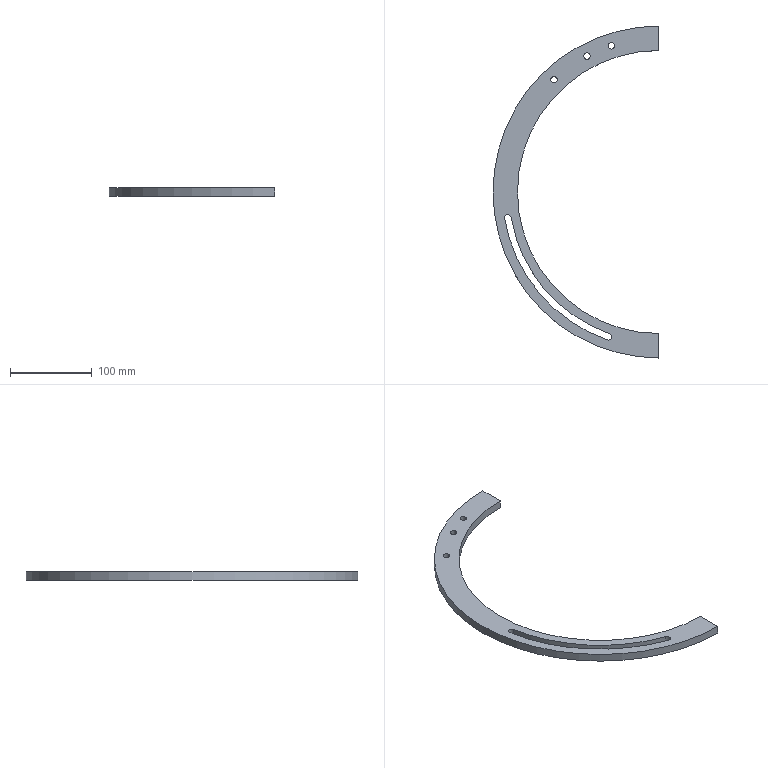Part | SolidWorks | features Cut 3, Extrusion 1 | 1 solid | 17 faces | box 203.295 x 406.59 x 10 mm | volume 159244 mm3 | cylinder 13 | plane 4 | commonest cylinder face diameters 8 x6 8.097 x3 346.59 x1 367.705 x1 383.898 x1 406.59 x1
STEP:
#1=CARTESIAN_POINT('',(229.318,361.783,-10.));
#2=VERTEX_POINT('',#1);
#3=CARTESIAN_POINT('',(237.318,361.783,-10.));
#4=VERTEX_POINT('',#3);
#5=CARTESIAN_POINT('',(233.318,361.783,-10.));
#6=DIRECTION('',(0.,0.,1.));
#7=DIRECTION('',(1.,0.,0.));
#8=AXIS2_PLACEMENT_3D('',#5,#6,#7);
#9=CIRCLE('',#8,4.);
#10=EDGE_CURVE('',#2,#4,#9,.T.);
#11=ORIENTED_EDGE('',*,*,#10,.F.);
#12=CARTESIAN_POINT('',(229.318,361.783,0.));
#13=VERTEX_POINT('',#12);
#14=CARTESIAN_POINT('',(229.318,361.783,-10.));
#15=DIRECTION('',(0.,0.,1.));
#16=VECTOR('',#15,1000.);
#17=LINE('',#14,#16);
#18=EDGE_CURVE('',#2,#13,#17,.T.);
#19=ORIENTED_EDGE('',*,*,#18,.T.);
#20=CARTESIAN_POINT('',(237.318,361.783,0.));
#21=VERTEX_POINT('',#20);
#22=CARTESIAN_POINT('',(233.318,361.783,0.));
#23=DIRECTION('',(0.,0.,1.));
#24=DIRECTION('',(1.,0.,0.));
#25=AXIS2_PLACEMENT_3D('',#22,#23,#24);
#26=CIRCLE('',#25,4.);
#27=EDGE_CURVE('',#13,#21,#26,.T.);
#28=ORIENTED_EDGE('',*,*,#27,.T.);
#29=CARTESIAN_POINT('',(237.318,361.783,-10.));
#30=DIRECTION('',(0.,0.,1.));
#31=VECTOR('',#30,1000.);
#32=LINE('',#29,#31);
#33=EDGE_CURVE('',#4,#21,#32,.T.);
#34=ORIENTED_EDGE('',*,*,#33,.F.);
#35=EDGE_LOOP('',(#11,#19,#28,#34));
#36=FACE_OUTER_BOUND('',#35,.T.);
#37=CARTESIAN_POINT('',(233.318,361.783,-10.));
#38=DIRECTION('',(0.,0.,1.));
#39=DIRECTION('',(1.,0.,0.));
#40=AXIS2_PLACEMENT_3D('',#37,#38,#39);
#41=CYLINDRICAL_SURFACE('',#40,4.);
#42=ADVANCED_FACE('',(#36),#41,.F.);
#43=CARTESIAN_POINT('',(199.412,349.105,-10.));
#44=VERTEX_POINT('',#43);
#45=CARTESIAN_POINT('',(207.412,349.105,-10.));
#46=VERTEX_POINT('',#45);
#47=CARTESIAN_POINT('',(203.412,349.105,-10.));
#48=DIRECTION('',(0.,0.,1.));
#49=DIRECTION('',(1.,0.,0.));
#50=AXIS2_PLACEMENT_3D('',#47,#48,#49);
#51=CIRCLE('',#50,4.);
#52=EDGE_CURVE('',#44,#46,#51,.T.);
#53=ORIENTED_EDGE('',*,*,#52,.F.);
#54=CARTESIAN_POINT('',(199.412,349.105,0.));
#55=VERTEX_POINT('',#54);
#56=CARTESIAN_POINT('',(199.412,349.105,-10.));
#57=DIRECTION('',(0.,0.,1.));
#58=VECTOR('',#57,1000.);
#59=LINE('',#56,#58);
#60=EDGE_CURVE('',#44,#55,#59,.T.);
#61=ORIENTED_EDGE('',*,*,#60,.T.);
#62=CARTESIAN_POINT('',(207.412,349.105,0.));
#63=VERTEX_POINT('',#62);
#64=CARTESIAN_POINT('',(203.412,349.105,0.));
#65=DIRECTION('',(0.,0.,1.));
#66=DIRECTION('',(1.,0.,0.));
#67=AXIS2_PLACEMENT_3D('',#64,#65,#66);
#68=CIRCLE('',#67,4.);
#69=EDGE_CURVE('',#55,#63,#68,.T.);
#70=ORIENTED_EDGE('',*,*,#69,.T.);
#71=CARTESIAN_POINT('',(207.412,349.105,-10.));
#72=DIRECTION('',(0.,0.,1.));
#73=VECTOR('',#72,1000.);
#74=LINE('',#71,#73);
#75=EDGE_CURVE('',#46,#63,#74,.T.);
#76=ORIENTED_EDGE('',*,*,#75,.F.);
#77=EDGE_LOOP('',(#53,#61,#70,#76));
#78=FACE_OUTER_BOUND('',#77,.T.);
#79=CARTESIAN_POINT('',(203.412,349.105,-10.));
#80=DIRECTION('',(0.,0.,1.));
#81=DIRECTION('',(1.,0.,0.));
#82=AXIS2_PLACEMENT_3D('',#79,#80,#81);
#83=CYLINDRICAL_SURFACE('',#82,4.);
#84=ADVANCED_FACE('',(#78),#83,.F.);
#85=CARTESIAN_POINT('',(158.898,320.188,-10.));
#86=VERTEX_POINT('',#85);
#87=CARTESIAN_POINT('',(166.898,320.188,-10.));
#88=VERTEX_POINT('',#87);
#89=CARTESIAN_POINT('',(162.898,320.188,-10.));
#90=DIRECTION('',(0.,0.,1.));
#91=DIRECTION('',(1.,0.,0.));
#92=AXIS2_PLACEMENT_3D('',#89,#90,#91);
#93=CIRCLE('',#92,4.);
#94=EDGE_CURVE('',#86,#88,#93,.T.);
#95=ORIENTED_EDGE('',*,*,#94,.F.);
#96=CARTESIAN_POINT('',(158.898,320.188,0.));
#97=VERTEX_POINT('',#96);
#98=CARTESIAN_POINT('',(158.898,320.188,-10.));
#99=DIRECTION('',(0.,0.,1.));
#100=VECTOR('',#99,1000.);
#101=LINE('',#98,#100);
#102=EDGE_CURVE('',#86,#97,#101,.T.);
#103=ORIENTED_EDGE('',*,*,#102,.T.);
#104=CARTESIAN_POINT('',(166.898,320.188,0.));
#105=VERTEX_POINT('',#104);
#106=CARTESIAN_POINT('',(162.898,320.188,0.));
#107=DIRECTION('',(0.,0.,1.));
#108=DIRECTION('',(1.,0.,0.));
#109=AXIS2_PLACEMENT_3D('',#106,#107,#108);
#110=CIRCLE('',#109,4.);
#111=EDGE_CURVE('',#97,#105,#110,.T.);
#112=ORIENTED_EDGE('',*,*,#111,.T.);
#113=CARTESIAN_POINT('',(166.898,320.188,-10.));
#114=DIRECTION('',(0.,0.,1.));
#115=VECTOR('',#114,1000.);
#116=LINE('',#113,#115);
#117=EDGE_CURVE('',#88,#105,#116,.T.);
#118=ORIENTED_EDGE('',*,*,#117,.F.);
#119=EDGE_LOOP('',(#95,#103,#112,#118));
#120=FACE_OUTER_BOUND('',#119,.T.);
#121=CARTESIAN_POINT('',(162.898,320.188,-10.));
#122=DIRECTION('',(0.,0.,1.));
#123=DIRECTION('',(1.,0.,0.));
#124=AXIS2_PLACEMENT_3D('',#121,#122,#123);
#125=CYLINDRICAL_SURFACE('',#124,4.);
#126=ADVANCED_FACE('',(#120),#125,.F.);
#127=CARTESIAN_POINT('',(110.405,151.499,0.));
#128=VERTEX_POINT('',#127);
#129=CARTESIAN_POINT('',(102.367,150.812,0.));
#130=VERTEX_POINT('',#129);
#131=CARTESIAN_POINT('',(106.416,150.812,0.));
#132=DIRECTION('',(0.,0.,1.));
#133=DIRECTION('',(1.,0.,0.));
#134=AXIS2_PLACEMENT_3D('',#131,#132,#133);
#135=CIRCLE('',#134,4.048);
#136=EDGE_CURVE('',#128,#130,#135,.T.);
#137=ORIENTED_EDGE('',*,*,#136,.T.);
#138=CARTESIAN_POINT('',(102.367,150.812,-10.));
#139=VERTEX_POINT('',#138);
#140=CARTESIAN_POINT('',(102.367,150.812,175.));
#141=DIRECTION('',(0.,0.,-1.));
#142=VECTOR('',#141,1000.);
#143=LINE('',#140,#142);
#144=EDGE_CURVE('',#130,#139,#143,.T.);
#145=ORIENTED_EDGE('',*,*,#144,.T.);
#146=CARTESIAN_POINT('',(110.405,151.499,-10.));
#147=VERTEX_POINT('',#146);
#148=CARTESIAN_POINT('',(106.416,150.812,-10.));
#149=DIRECTION('',(0.,0.,-1.));
#150=DIRECTION('',(-1.,0.,0.));
#151=AXIS2_PLACEMENT_3D('',#148,#149,#150);
#152=CIRCLE('',#151,4.048);
#153=EDGE_CURVE('',#139,#147,#152,.T.);
#154=ORIENTED_EDGE('',*,*,#153,.T.);
#155=CARTESIAN_POINT('',(110.405,151.499,175.));
#156=DIRECTION('',(0.,0.,-1.));
#157=VECTOR('',#156,1000.);
#158=LINE('',#155,#157);
#159=EDGE_CURVE('',#128,#147,#158,.T.);
#160=ORIENTED_EDGE('',*,*,#159,.F.);
#161=EDGE_LOOP('',(#137,#145,#154,#160));
#162=FACE_OUTER_BOUND('',#161,.T.);
#163=CARTESIAN_POINT('',(106.416,150.812,175.));
#164=DIRECTION('',(0.,0.,-1.));
#165=DIRECTION('',(-1.,0.,0.));
#166=AXIS2_PLACEMENT_3D('',#163,#164,#165);
#167=CYLINDRICAL_SURFACE('',#166,4.048);
#168=ADVANCED_FACE('',(#162),#167,.F.);
#169=CARTESIAN_POINT('',(291.585,-20.564,0.));
#170=VERTEX_POINT('',#169);
#171=CARTESIAN_POINT('',(291.585,-20.564,-10.));
#172=VERTEX_POINT('',#171);
#173=CARTESIAN_POINT('',(291.585,-20.564,-10.));
#174=DIRECTION('',(0.,0.,-1.));
#175=VECTOR('',#174,1000.);
#176=LINE('',#173,#175);
#177=EDGE_CURVE('',#170,#172,#176,.T.);
#178=ORIENTED_EDGE('',*,*,#177,.F.);
#179=CARTESIAN_POINT('',(291.585,386.026,0.));
#180=VERTEX_POINT('',#179);
#181=CARTESIAN_POINT('',(291.585,182.731,0.));
#182=DIRECTION('',(0.,0.,1.));
#183=DIRECTION('',(1.,0.,0.));
#184=AXIS2_PLACEMENT_3D('',#181,#182,#183);
#185=CIRCLE('',#184,203.295);
#186=EDGE_CURVE('',#180,#170,#185,.T.);
#187=ORIENTED_EDGE('',*,*,#186,.F.);
#188=CARTESIAN_POINT('',(291.585,386.026,-10.));
#189=VERTEX_POINT('',#188);
#190=CARTESIAN_POINT('',(291.585,386.026,-10.));
#191=DIRECTION('',(0.,0.,1.));
#192=VECTOR('',#191,1000.);
#193=LINE('',#190,#192);
#194=EDGE_CURVE('',#189,#180,#193,.T.);
#195=ORIENTED_EDGE('',*,*,#194,.F.);
#196=CARTESIAN_POINT('',(291.585,182.731,-10.));
#197=DIRECTION('',(0.,0.,1.));
#198=DIRECTION('',(1.,0.,0.));
#199=AXIS2_PLACEMENT_3D('',#196,#197,#198);
#200=CIRCLE('',#199,203.295);
#201=EDGE_CURVE('',#189,#172,#200,.T.);
#202=ORIENTED_EDGE('',*,*,#201,.T.);
#203=EDGE_LOOP('',(#178,#187,#195,#202));
#204=FACE_OUTER_BOUND('',#203,.T.);
#205=CARTESIAN_POINT('',(291.585,182.731,-10.));
#206=DIRECTION('',(0.,0.,1.));
#207=DIRECTION('',(1.,0.,0.));
#208=AXIS2_PLACEMENT_3D('',#205,#206,#207);
#209=CYLINDRICAL_SURFACE('',#208,203.295);
#210=ADVANCED_FACE('',(#204),#209,.T.);
#211=CARTESIAN_POINT('',(233.318,361.783,-10.));
#212=DIRECTION('',(0.,0.,1.));
#213=DIRECTION('',(1.,0.,0.));
#214=AXIS2_PLACEMENT_3D('',#211,#212,#213);
#215=CIRCLE('',#214,4.);
#216=EDGE_CURVE('',#4,#2,#215,.T.);
#217=ORIENTED_EDGE('',*,*,#216,.T.);
#218=ORIENTED_EDGE('',*,*,#10,.T.);
#219=EDGE_LOOP('',(#217,#218));
#220=FACE_BOUND('',#219,.T.);
#221=CARTESIAN_POINT('',(203.412,349.105,-10.));
#222=DIRECTION('',(0.,0.,1.));
#223=DIRECTION('',(1.,0.,0.));
#224=AXIS2_PLACEMENT_3D('',#221,#222,#223);
#225=CIRCLE('',#224,4.);
#226=EDGE_CURVE('',#46,#44,#225,.T.);
#227=ORIENTED_EDGE('',*,*,#226,.T.);
#228=ORIENTED_EDGE('',*,*,#52,.T.);
#229=EDGE_LOOP('',(#227,#228));
#230=FACE_BOUND('',#229,.T.);
#231=CARTESIAN_POINT('',(162.898,320.188,-10.));
#232=DIRECTION('',(0.,0.,1.));
#233=DIRECTION('',(1.,0.,0.));
#234=AXIS2_PLACEMENT_3D('',#231,#232,#233);
#235=CIRCLE('',#234,4.);
#236=EDGE_CURVE('',#88,#86,#235,.T.);
#237=ORIENTED_EDGE('',*,*,#236,.T.);
#238=ORIENTED_EDGE('',*,*,#94,.T.);
#239=EDGE_LOOP('',(#237,#238));
#240=FACE_BOUND('',#239,.T.);
#241=CARTESIAN_POINT('',(228.398,1.48,-10.));
#242=VERTEX_POINT('',#241);
#243=CARTESIAN_POINT('',(102.426,150.124,-10.));
#244=VERTEX_POINT('',#243);
#245=CARTESIAN_POINT('',(291.585,182.731,-10.));
#246=DIRECTION('',(0.,0.,-1.));
#247=DIRECTION('',(-1.,0.,0.));
#248=AXIS2_PLACEMENT_3D('',#245,#246,#247);
#249=CIRCLE('',#248,191.949);
#250=EDGE_CURVE('',#242,#244,#249,.T.);
#251=ORIENTED_EDGE('',*,*,#250,.F.);
#252=CARTESIAN_POINT('',(231.063,9.125,-10.));
#253=VERTEX_POINT('',#252);
#254=CARTESIAN_POINT('',(229.731,5.303,-10.));
#255=DIRECTION('',(0.,0.,-1.));
#256=DIRECTION('',(-1.,0.,0.));
#257=AXIS2_PLACEMENT_3D('',#254,#255,#256);
#258=CIRCLE('',#257,4.048);
#259=EDGE_CURVE('',#253,#242,#258,.T.);
#260=ORIENTED_EDGE('',*,*,#259,.F.);
#261=CARTESIAN_POINT('',(291.585,182.731,-10.));
#262=DIRECTION('',(0.,0.,1.));
#263=DIRECTION('',(-1.,0.,0.));
#264=AXIS2_PLACEMENT_3D('',#261,#262,#263);
#265=CIRCLE('',#264,183.852);
#266=EDGE_CURVE('',#147,#253,#265,.T.);
#267=ORIENTED_EDGE('',*,*,#266,.F.);
#268=ORIENTED_EDGE('',*,*,#153,.F.);
#269=CARTESIAN_POINT('',(106.416,150.812,-10.));
#270=DIRECTION('',(0.,0.,-1.));
#271=DIRECTION('',(-1.,0.,0.));
#272=AXIS2_PLACEMENT_3D('',#269,#270,#271);
#273=CIRCLE('',#272,4.048);
#274=EDGE_CURVE('',#244,#139,#273,.T.);
#275=ORIENTED_EDGE('',*,*,#274,.F.);
#276=EDGE_LOOP('',(#251,#260,#267,#268,#275));
#277=FACE_BOUND('',#276,.T.);
#278=CARTESIAN_POINT('',(291.585,356.026,-10.));
#279=VERTEX_POINT('',#278);
#280=CARTESIAN_POINT('',(291.585,9.436,-10.));
#281=VERTEX_POINT('',#280);
#282=CARTESIAN_POINT('',(291.585,182.731,-10.));
#283=DIRECTION('',(0.,0.,1.));
#284=DIRECTION('',(1.,0.,0.));
#285=AXIS2_PLACEMENT_3D('',#282,#283,#284);
#286=CIRCLE('',#285,173.295);
#287=EDGE_CURVE('',#279,#281,#286,.T.);
#288=ORIENTED_EDGE('',*,*,#287,.T.);
#289=CARTESIAN_POINT('',(291.585,9.436,-10.));
#290=DIRECTION('',(0.,1.,0.));
#291=VECTOR('',#290,1000.);
#292=LINE('',#289,#291);
#293=EDGE_CURVE('',#172,#281,#292,.T.);
#294=ORIENTED_EDGE('',*,*,#293,.F.);
#295=ORIENTED_EDGE('',*,*,#201,.F.);
#296=CARTESIAN_POINT('',(291.585,356.026,-10.));
#297=DIRECTION('',(0.,1.,0.));
#298=VECTOR('',#297,1000.);
#299=LINE('',#296,#298);
#300=EDGE_CURVE('',#279,#189,#299,.T.);
#301=ORIENTED_EDGE('',*,*,#300,.F.);
#302=EDGE_LOOP('',(#288,#294,#295,#301));
#303=FACE_OUTER_BOUND('',#302,.T.);
#304=CARTESIAN_POINT('',(291.585,182.731,-10.));
#305=DIRECTION('',(0.,0.,1.));
#306=DIRECTION('',(1.,0.,0.));
#307=AXIS2_PLACEMENT_3D('',#304,#305,#306);
#308=PLANE('',#307);
#309=ADVANCED_FACE('',(#220,#230,#240,#277,#303),#308,.F.);
#310=CARTESIAN_POINT('',(233.318,361.783,0.));
#311=DIRECTION('',(0.,0.,1.));
#312=DIRECTION('',(1.,0.,0.));
#313=AXIS2_PLACEMENT_3D('',#310,#311,#312);
#314=CIRCLE('',#313,4.);
#315=EDGE_CURVE('',#21,#13,#314,.T.);
#316=ORIENTED_EDGE('',*,*,#315,.F.);
#317=ORIENTED_EDGE('',*,*,#27,.F.);
#318=EDGE_LOOP('',(#316,#317));
#319=FACE_BOUND('',#318,.T.);
#320=CARTESIAN_POINT('',(203.412,349.105,0.));
#321=DIRECTION('',(0.,0.,1.));
#322=DIRECTION('',(1.,0.,0.));
#323=AXIS2_PLACEMENT_3D('',#320,#321,#322);
#324=CIRCLE('',#323,4.);
#325=EDGE_CURVE('',#63,#55,#324,.T.);
#326=ORIENTED_EDGE('',*,*,#325,.F.);
#327=ORIENTED_EDGE('',*,*,#69,.F.);
#328=EDGE_LOOP('',(#326,#327));
#329=FACE_BOUND('',#328,.T.);
#330=CARTESIAN_POINT('',(162.898,320.188,0.));
#331=DIRECTION('',(0.,0.,1.));
#332=DIRECTION('',(1.,0.,0.));
#333=AXIS2_PLACEMENT_3D('',#330,#331,#332);
#334=CIRCLE('',#333,4.);
#335=EDGE_CURVE('',#105,#97,#334,.T.);
#336=ORIENTED_EDGE('',*,*,#335,.F.);
#337=ORIENTED_EDGE('',*,*,#111,.F.);
#338=EDGE_LOOP('',(#336,#337));
#339=FACE_BOUND('',#338,.T.);
#340=CARTESIAN_POINT('',(228.398,1.48,0.));
#341=VERTEX_POINT('',#340);
#342=CARTESIAN_POINT('',(231.063,9.125,0.));
#343=VERTEX_POINT('',#342);
#344=CARTESIAN_POINT('',(229.731,5.303,0.));
#345=DIRECTION('',(0.,0.,1.));
#346=DIRECTION('',(1.,0.,0.));
#347=AXIS2_PLACEMENT_3D('',#344,#345,#346);
#348=CIRCLE('',#347,4.048);
#349=EDGE_CURVE('',#341,#343,#348,.T.);
#350=ORIENTED_EDGE('',*,*,#349,.F.);
#351=CARTESIAN_POINT('',(102.426,150.124,0.));
#352=VERTEX_POINT('',#351);
#353=CARTESIAN_POINT('',(291.585,182.731,0.));
#354=DIRECTION('',(0.,0.,1.));
#355=DIRECTION('',(1.,0.,0.));
#356=AXIS2_PLACEMENT_3D('',#353,#354,#355);
#357=CIRCLE('',#356,191.949);
#358=EDGE_CURVE('',#352,#341,#357,.T.);
#359=ORIENTED_EDGE('',*,*,#358,.F.);
#360=CARTESIAN_POINT('',(106.416,150.812,0.));
#361=DIRECTION('',(0.,0.,1.));
#362=DIRECTION('',(1.,0.,0.));
#363=AXIS2_PLACEMENT_3D('',#360,#361,#362);
#364=CIRCLE('',#363,4.048);
#365=EDGE_CURVE('',#130,#352,#364,.T.);
#366=ORIENTED_EDGE('',*,*,#365,.F.);
#367=ORIENTED_EDGE('',*,*,#136,.F.);
#368=CARTESIAN_POINT('',(291.585,182.731,0.));
#369=DIRECTION('',(0.,0.,-1.));
#370=DIRECTION('',(1.,0.,0.));
#371=AXIS2_PLACEMENT_3D('',#368,#369,#370);
#372=CIRCLE('',#371,183.852);
#373=EDGE_CURVE('',#343,#128,#372,.T.);
#374=ORIENTED_EDGE('',*,*,#373,.F.);
#375=EDGE_LOOP('',(#350,#359,#366,#367,#374));
#376=FACE_BOUND('',#375,.T.);
#377=CARTESIAN_POINT('',(291.585,9.436,0.));
#378=VERTEX_POINT('',#377);
#379=CARTESIAN_POINT('',(291.585,182.731,0.));
#380=DIRECTION('',(0.,-1.,0.));
#381=VECTOR('',#380,1000.);
#382=LINE('',#379,#381);
#383=EDGE_CURVE('',#378,#170,#382,.T.);
#384=ORIENTED_EDGE('',*,*,#383,.F.);
#385=CARTESIAN_POINT('',(291.585,356.026,0.));
#386=VERTEX_POINT('',#385);
#387=CARTESIAN_POINT('',(291.585,182.731,0.));
#388=DIRECTION('',(0.,0.,1.));
#389=DIRECTION('',(1.,0.,0.));
#390=AXIS2_PLACEMENT_3D('',#387,#388,#389);
#391=CIRCLE('',#390,173.295);
#392=EDGE_CURVE('',#386,#378,#391,.T.);
#393=ORIENTED_EDGE('',*,*,#392,.F.);
#394=CARTESIAN_POINT('',(291.585,182.731,0.));
#395=DIRECTION('',(0.,-1.,0.));
#396=VECTOR('',#395,1000.);
#397=LINE('',#394,#396);
#398=EDGE_CURVE('',#180,#386,#397,.T.);
#399=ORIENTED_EDGE('',*,*,#398,.F.);
#400=ORIENTED_EDGE('',*,*,#186,.T.);
#401=EDGE_LOOP('',(#384,#393,#399,#400));
#402=FACE_OUTER_BOUND('',#401,.T.);
#403=CARTESIAN_POINT('',(291.585,182.731,0.));
#404=DIRECTION('',(0.,0.,1.));
#405=DIRECTION('',(1.,0.,0.));
#406=AXIS2_PLACEMENT_3D('',#403,#404,#405);
#407=PLANE('',#406);
#408=ADVANCED_FACE('',(#319,#329,#339,#376,#402),#407,.T.);
#409=ORIENTED_EDGE('',*,*,#392,.T.);
#410=CARTESIAN_POINT('',(291.585,9.436,-10.));
#411=DIRECTION('',(0.,0.,-1.));
#412=VECTOR('',#411,1000.);
#413=LINE('',#410,#412);
#414=EDGE_CURVE('',#378,#281,#413,.T.);
#415=ORIENTED_EDGE('',*,*,#414,.T.);
#416=ORIENTED_EDGE('',*,*,#287,.F.);
#417=CARTESIAN_POINT('',(291.585,356.026,-10.));
#418=DIRECTION('',(0.,0.,1.));
#419=VECTOR('',#418,1000.);
#420=LINE('',#417,#419);
#421=EDGE_CURVE('',#279,#386,#420,.T.);
#422=ORIENTED_EDGE('',*,*,#421,.T.);
#423=EDGE_LOOP('',(#409,#415,#416,#422));
#424=FACE_OUTER_BOUND('',#423,.T.);
#425=CARTESIAN_POINT('',(291.585,182.731,-10.));
#426=DIRECTION('',(0.,0.,1.));
#427=DIRECTION('',(1.,0.,0.));
#428=AXIS2_PLACEMENT_3D('',#425,#426,#427);
#429=CYLINDRICAL_SURFACE('',#428,173.295);
#430=ADVANCED_FACE('',(#424),#429,.F.);
#431=ORIENTED_EDGE('',*,*,#194,.T.);
#432=ORIENTED_EDGE('',*,*,#398,.T.);
#433=ORIENTED_EDGE('',*,*,#421,.F.);
#434=ORIENTED_EDGE('',*,*,#300,.T.);
#435=EDGE_LOOP('',(#431,#432,#433,#434));
#436=FACE_OUTER_BOUND('',#435,.T.);
#437=CARTESIAN_POINT('',(291.585,356.026,175.));
#438=DIRECTION('',(-1.,0.,0.));
#439=DIRECTION('',(0.,0.,1.));
#440=AXIS2_PLACEMENT_3D('',#437,#438,#439);
#441=PLANE('',#440);
#442=ADVANCED_FACE('',(#436),#441,.F.);
#443=ORIENTED_EDGE('',*,*,#177,.T.);
#444=ORIENTED_EDGE('',*,*,#293,.T.);
#445=ORIENTED_EDGE('',*,*,#414,.F.);
#446=ORIENTED_EDGE('',*,*,#383,.T.);
#447=EDGE_LOOP('',(#443,#444,#445,#446));
#448=FACE_OUTER_BOUND('',#447,.T.);
#449=CARTESIAN_POINT('',(291.585,9.436,175.));
#450=DIRECTION('',(-1.,0.,0.));
#451=DIRECTION('',(0.,0.,1.));
#452=AXIS2_PLACEMENT_3D('',#449,#450,#451);
#453=PLANE('',#452);
#454=ADVANCED_FACE('',(#448),#453,.F.);
#455=ORIENTED_EDGE('',*,*,#349,.T.);
#456=CARTESIAN_POINT('',(231.063,9.125,175.));
#457=DIRECTION('',(0.,0.,-1.));
#458=VECTOR('',#457,1000.);
#459=LINE('',#456,#458);
#460=EDGE_CURVE('',#343,#253,#459,.T.);
#461=ORIENTED_EDGE('',*,*,#460,.T.);
#462=ORIENTED_EDGE('',*,*,#259,.T.);
#463=CARTESIAN_POINT('',(228.398,1.48,175.));
#464=DIRECTION('',(0.,0.,-1.));
#465=VECTOR('',#464,1000.);
#466=LINE('',#463,#465);
#467=EDGE_CURVE('',#341,#242,#466,.T.);
#468=ORIENTED_EDGE('',*,*,#467,.F.);
#469=EDGE_LOOP('',(#455,#461,#462,#468));
#470=FACE_OUTER_BOUND('',#469,.T.);
#471=CARTESIAN_POINT('',(229.731,5.303,175.));
#472=DIRECTION('',(0.,0.,-1.));
#473=DIRECTION('',(-1.,0.,0.));
#474=AXIS2_PLACEMENT_3D('',#471,#472,#473);
#475=CYLINDRICAL_SURFACE('',#474,4.048);
#476=ADVANCED_FACE('',(#470),#475,.F.);
#477=ORIENTED_EDGE('',*,*,#373,.T.);
#478=ORIENTED_EDGE('',*,*,#159,.T.);
#479=ORIENTED_EDGE('',*,*,#266,.T.);
#480=ORIENTED_EDGE('',*,*,#460,.F.);
#481=EDGE_LOOP('',(#477,#478,#479,#480));
#482=FACE_OUTER_BOUND('',#481,.T.);
#483=CARTESIAN_POINT('',(291.585,182.731,175.));
#484=DIRECTION('',(0.,0.,-1.));
#485=DIRECTION('',(-1.,0.,0.));
#486=AXIS2_PLACEMENT_3D('',#483,#484,#485);
#487=CYLINDRICAL_SURFACE('',#486,183.852);
#488=ADVANCED_FACE('',(#482),#487,.T.);
#489=ORIENTED_EDGE('',*,*,#144,.F.);
#490=ORIENTED_EDGE('',*,*,#365,.T.);
#491=CARTESIAN_POINT('',(102.426,150.124,175.));
#492=DIRECTION('',(0.,0.,-1.));
#493=VECTOR('',#492,1000.);
#494=LINE('',#491,#493);
#495=EDGE_CURVE('',#352,#244,#494,.T.);
#496=ORIENTED_EDGE('',*,*,#495,.T.);
#497=ORIENTED_EDGE('',*,*,#274,.T.);
#498=EDGE_LOOP('',(#489,#490,#496,#497));
#499=FACE_OUTER_BOUND('',#498,.T.);
#500=CARTESIAN_POINT('',(106.416,150.812,175.));
#501=DIRECTION('',(0.,0.,-1.));
#502=DIRECTION('',(-1.,0.,0.));
#503=AXIS2_PLACEMENT_3D('',#500,#501,#502);
#504=CYLINDRICAL_SURFACE('',#503,4.048);
#505=ADVANCED_FACE('',(#499),#504,.F.);
#506=ORIENTED_EDGE('',*,*,#358,.T.);
#507=ORIENTED_EDGE('',*,*,#467,.T.);
#508=ORIENTED_EDGE('',*,*,#250,.T.);
#509=ORIENTED_EDGE('',*,*,#495,.F.);
#510=EDGE_LOOP('',(#506,#507,#508,#509));
#511=FACE_OUTER_BOUND('',#510,.T.);
#512=CARTESIAN_POINT('',(291.585,182.731,175.));
#513=DIRECTION('',(0.,0.,-1.));
#514=DIRECTION('',(-1.,0.,0.));
#515=AXIS2_PLACEMENT_3D('',#512,#513,#514);
#516=CYLINDRICAL_SURFACE('',#515,191.949);
#517=ADVANCED_FACE('',(#511),#516,.F.);
#518=ORIENTED_EDGE('',*,*,#102,.F.);
#519=ORIENTED_EDGE('',*,*,#236,.F.);
#520=ORIENTED_EDGE('',*,*,#117,.T.);
#521=ORIENTED_EDGE('',*,*,#335,.T.);
#522=EDGE_LOOP('',(#518,#519,#520,#521));
#523=FACE_OUTER_BOUND('',#522,.T.);
#524=CARTESIAN_POINT('',(162.898,320.188,-10.));
#525=DIRECTION('',(0.,0.,1.));
#526=DIRECTION('',(1.,0.,0.));
#527=AXIS2_PLACEMENT_3D('',#524,#525,#526);
#528=CYLINDRICAL_SURFACE('',#527,4.);
#529=ADVANCED_FACE('',(#523),#528,.F.);
#530=ORIENTED_EDGE('',*,*,#60,.F.);
#531=ORIENTED_EDGE('',*,*,#226,.F.);
#532=ORIENTED_EDGE('',*,*,#75,.T.);
#533=ORIENTED_EDGE('',*,*,#325,.T.);
#534=EDGE_LOOP('',(#530,#531,#532,#533));
#535=FACE_OUTER_BOUND('',#534,.T.);
#536=CARTESIAN_POINT('',(203.412,349.105,-10.));
#537=DIRECTION('',(0.,0.,1.));
#538=DIRECTION('',(1.,0.,0.));
#539=AXIS2_PLACEMENT_3D('',#536,#537,#538);
#540=CYLINDRICAL_SURFACE('',#539,4.);
#541=ADVANCED_FACE('',(#535),#540,.F.);
#542=ORIENTED_EDGE('',*,*,#18,.F.);
#543=ORIENTED_EDGE('',*,*,#216,.F.);
#544=ORIENTED_EDGE('',*,*,#33,.T.);
#545=ORIENTED_EDGE('',*,*,#315,.T.);
#546=EDGE_LOOP('',(#542,#543,#544,#545));
#547=FACE_OUTER_BOUND('',#546,.T.);
#548=CARTESIAN_POINT('',(233.318,361.783,-10.));
#549=DIRECTION('',(0.,0.,1.));
#550=DIRECTION('',(1.,0.,0.));
#551=AXIS2_PLACEMENT_3D('',#548,#549,#550);
#552=CYLINDRICAL_SURFACE('',#551,4.);
#553=ADVANCED_FACE('',(#547),#552,.F.);
#554=CLOSED_SHELL('',(#42,#84,#126,#168,#210,#309,#408,#430,#442,#454,#476,#488,#505,#517,#529,#541,#553));
#555=MANIFOLD_SOLID_BREP('',#554);
#556=CARTESIAN_POINT('',(0.,0.,0.));
#557=DIRECTION('',(0.,0.,1.));
#558=DIRECTION('',(1.,0.,0.));
#559=AXIS2_PLACEMENT_3D('',#556,#557,#558);
#560=(LENGTH_UNIT()NAMED_UNIT(*)SI_UNIT(.MILLI.,.METRE.));
#561=UNCERTAINTY_MEASURE_WITH_UNIT(LENGTH_MEASURE(0.00001),#560,'','');
#562=(NAMED_UNIT(*)PLANE_ANGLE_UNIT()SI_UNIT($,.RADIAN.));
#563=(NAMED_UNIT(*)SI_UNIT($,.STERADIAN.)SOLID_ANGLE_UNIT());
#564=(GEOMETRIC_REPRESENTATION_CONTEXT(3)GLOBAL_UNCERTAINTY_ASSIGNED_CONTEXT((#561))GLOBAL_UNIT_ASSIGNED_CONTEXT((#560,#562,#563))REPRESENTATION_CONTEXT('',''));
#565=ADVANCED_BREP_SHAPE_REPRESENTATION('',(#555,#559),#564);